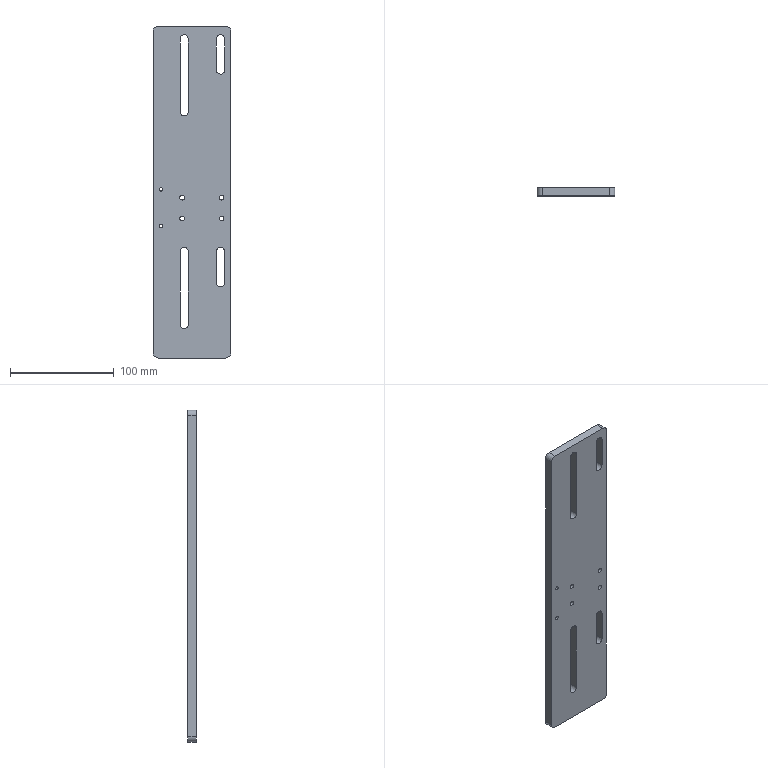Part | STEP file | 0246_215_Plate | 1 solid | 42 faces | box 75 x 8 x 320 mm | volume 176774 mm3 | cylinder 28 | plane 14 | commonest cylinder face diameters 8 x12 4.5 x8 3.3 x4 10 x4